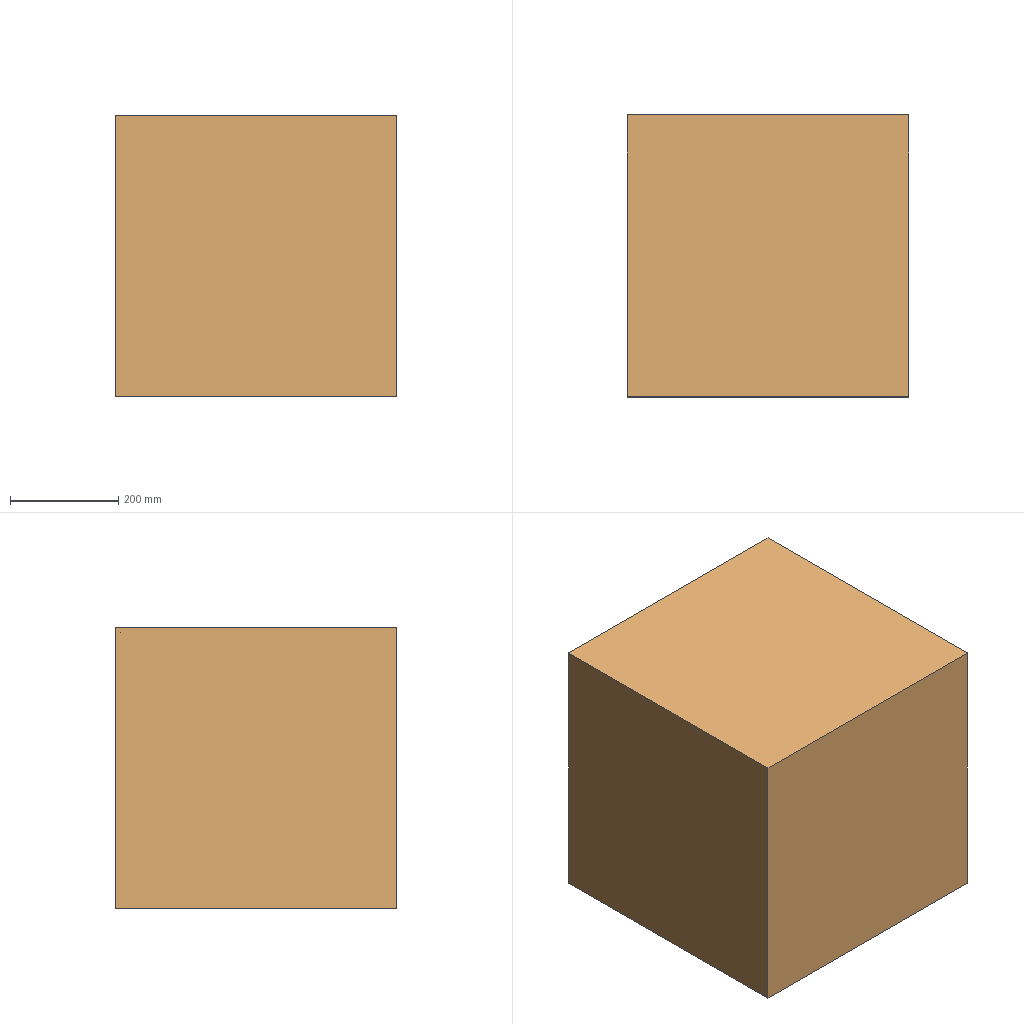Assembly | SolidWorks | 12 different items | 12 placed | box 520 x 520 x 520 mm
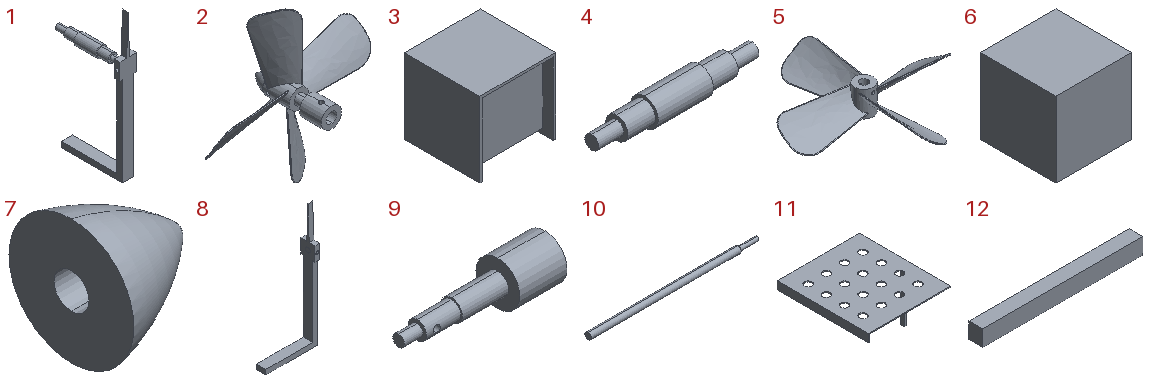Parts list (item | name | quantity | parent item | size | volume | features):
1 | (subassembly) | x1 | - | 30 x 126.1 x 261.431 mm | 85537 mm3 | -
2 | (subassembly) | x1 | - | 146.733 x 70.903 x 146.733 mm | 21396 mm3 | -
3 | - | x1 | - | 60.365 x 60 x 59.674 mm | 146086 mm3 | features ICE 5, BaseBody 1
4 | - | x1 | in 1 | 116 x 20 x 20 mm | 23436 mm3 | features BaseBody 1
5 | - | x1 | in 2 | 147.93 x 147.93 x 25 mm | 13194 mm3 | features BaseBody 1
6 | - | x1 | - | 520 x 520 x 520 mm | 15406938 mm3 | features ICE 2, BaseBody 1
7 | - | x1 | in 2 | 15.4 x 17.8 x 17.8 mm | 1658 mm3 | features BaseBody 1
8 | - | x1 | in 1 | 110 x 30 x 261.431 mm | 62100 mm3 | features ICE 2, BaseBody 1
9 | - | x1 | in 2 | 63.5 x 19 x 19 mm | 6544 mm3 | features BaseBody 1
10 | - | x1 | - | 264.77 x 10 x 10 mm | 19287 mm3 | features BaseBody 1, ICE 1
11 | - | x1 | - | 450 x 500 x 305 mm | 1181124 mm3 | features ICE 3, BaseBody 2
12 | - | x1 | - | 500 x 43.66 x 50 mm | 1091500 mm3 | features BaseBody 1
Mates (type | each side: item.copy, entity, surface, feature):
DistanceDim | 11.1 face plane Input1 | 6.1 face plane Input1 | 2 times
Coincident | 8.1 face plane Input1 | 10.1 face plane Input1
Coincident | 9.1 face plane Input1 | 4.1 face plane Input1
Concentric | 9.1 face cylinder Input1 | 4.1 face cylinder Input1
Coincident | 6.1 face plane Input1 | 11.1 face plane Boss-Extrude2
Concentric | 8.1 face cylinder Input1 | 10.1 face cylinder Input1
Coincident | 6.1 face plane Input1 | 3.1 face plane Input1
DistanceDim | 6.1 face plane Input1 | 3.1 face plane Boss-Extrude3
DistanceDim | 6.1 face plane Input1 | 3.1 face plane Input1